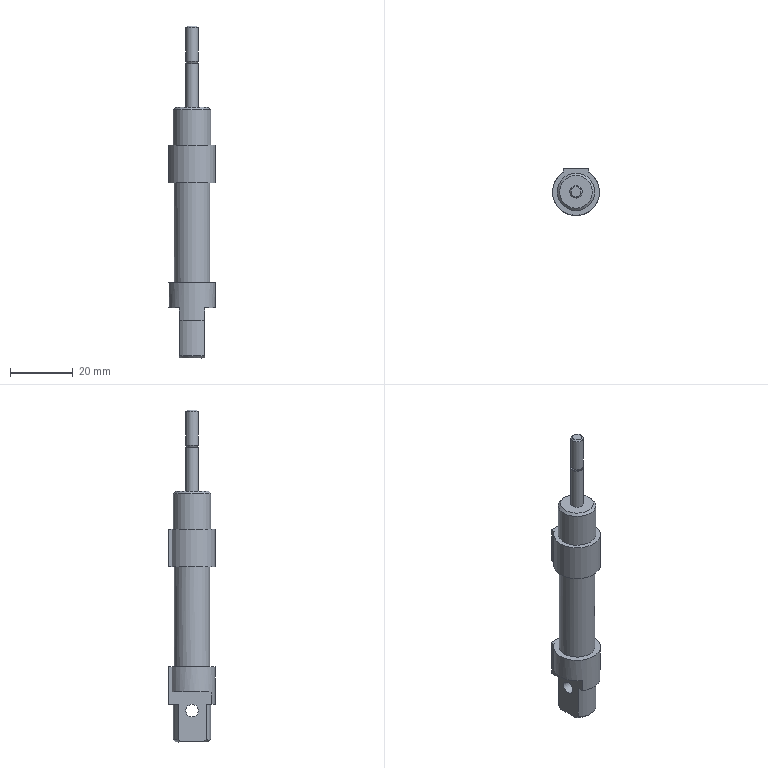Part | STEP file | 19183 DSNU-10-10-P-A | 2 solids | 44 faces | box 15 x 15 x 106 mm | volume 9040 mm3 | plane 23 | cylinder 14 | cone 7 | commonest cylinder face diameters 4 x4 12 x3 4.134 x2 10 x2 15 x2 11.3 x1